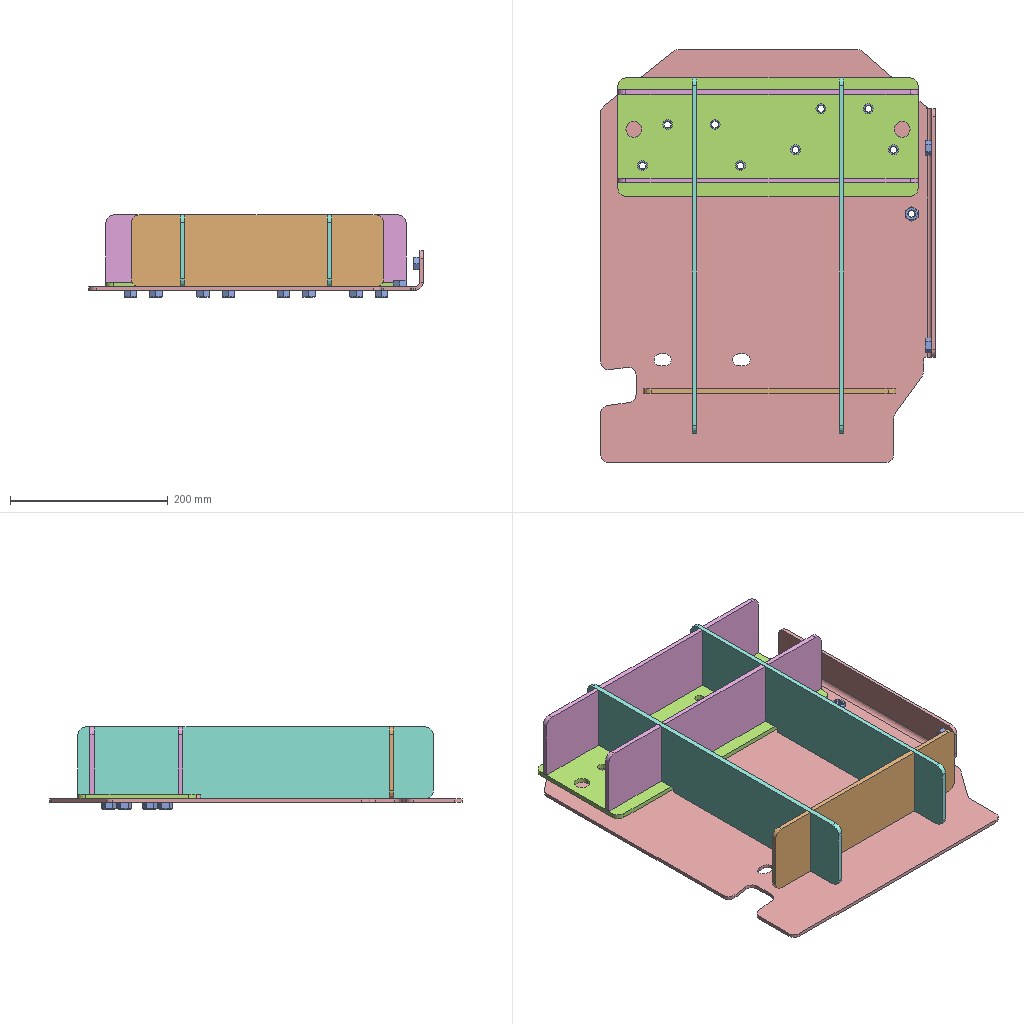Assembly | SolidWorks | 6 different items | 18 placed | box 424 x 523 x 104 mm
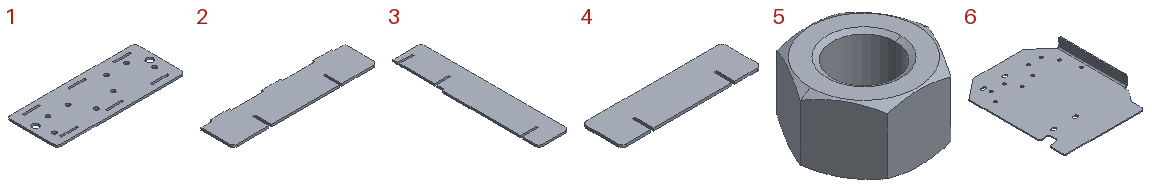Parts list (item | quantity | size | volume | features):
1 | x1 | 380 x 150 x 6 mm | 321025 mm3 | features FlatPattern 1, SMBaseFlange 1, SheetMetal 1
2 | x2 | 380 x 90.5 x 6 mm | 195432 mm3 | features FlatPattern 1, SMBaseFlange 1, SheetMetal 1
3 | x2 | 91 x 450 x 6 mm | 234874 mm3 | features FlatPattern 1, SMBaseFlange 1, SheetMetal 1
4 | x1 | 320 x 91 x 6 mm | 171145 mm3 | features Fillet 1, FlatPattern 1, SMBaseFlange 1, SheetMetal 1
5 | x11 | 27.713 x 24 x 14.8 mm | 5071 mm3 | features RevCut 2, Chamfer 1, Extrusion 1, LPattern 1
6 | x1 | 424 x 523 x 50 mm | 979518 mm3 | features EdgeFlange 1, Fillet 1, FlatPattern 1, ICE 1, SMBaseFlange 1, SheetMetal 1
Mates (type | each side: item.copy, entity, surface, feature):
Concentric | 6.1 face cylinder Base-Flange1 | 5.1 face cone EndChamfer
Coincident | 6.1 face plane Base-Flange1 | 5.1 face plane BaseNut
Parallel | 6.1 face plane Edge-Flange1 | 5.1 face plane BaseNut
Concentric | 6.1 face cylinder Cut-Extrude1 | 5.2 face cone EndChamfer
Coincident | 6.1 face plane Edge-Flange1 | 5.2 face plane BaseNut
Parallel | 6.1 face plane Edge-Flange1 | 5.2 face plane BaseNut
Concentric | 6.1 face cylinder Cut-Extrude1 | 5.3 face cone EndChamfer
Coincident | 6.1 face plane Edge-Flange1 | 5.3 face plane BaseNut
Parallel | 6.1 face plane Edge-Flange1 | 5.3 face plane BaseNut
Concentric | 6.1 face cylinder Base-Flange1 | 5.4 face cone EndChamfer
Coincident | 6.1 face plane Base-Flange1 | 5.4 face plane BaseNut
Parallel | 6.1 face plane Edge-Flange1 | 5.4 face plane BaseNut
Concentric | 6.1 face cylinder Base-Flange1 | 5.5 face cone EndChamfer
Coincident | 6.1 face plane Base-Flange1 | 5.5 face plane BaseNut
Concentric | 6.1 face cylinder Base-Flange1 | 5.6 face cone EndChamfer
Coincident | 6.1 face plane Base-Flange1 | 5.6 face plane BaseNut
Concentric | 6.1 face cylinder Base-Flange1 | 5.7 face cone EndChamfer
Coincident | 6.1 face plane Base-Flange1 | 5.7 face plane BaseNut
Concentric | 6.1 face cylinder Base-Flange1 | 5.8 face cone EndChamfer
Coincident | 6.1 face plane Base-Flange1 | 5.8 face plane BaseNut
Concentric | 6.1 face cylinder Base-Flange1 | 5.9 face cone EndChamfer
Coincident | 6.1 face plane Base-Flange1 | 5.9 face plane BaseNut
Concentric | 6.1 face cylinder Base-Flange1 | 5.10 face cone EndChamfer
Coincident | 6.1 face plane Base-Flange1 | 5.10 face plane BaseNut
Concentric | 6.1 face cylinder Base-Flange1 | 5.11 face cone EndChamfer
Coincident | 6.1 face plane Base-Flange1 | 5.11 face plane BaseNut
Parallel | 6.1 face plane Edge-Flange1 | 5.6 face plane BaseNut
Parallel | 6.1 face plane Edge-Flange1 | 5.5 face plane BaseNut
Parallel | 6.1 face plane Edge-Flange1 | 5.7 face plane BaseNut
Parallel | 6.1 face plane Edge-Flange1 | 5.8 face plane BaseNut
Parallel | 6.1 face plane Edge-Flange1 | 5.10 face plane BaseNut
Parallel | 6.1 face plane Edge-Flange1 | 5.9 face plane BaseNut
Parallel | 6.1 face plane Edge-Flange1 | 5.11 face plane BaseNut
InPlace | 6.1 face plane Base-Flange1 | 1.1 plane
InPlace | 2.1 plane | assembly plane
InPlace | 3.1 plane | assembly plane
InPlace | 4.1 plane | assembly plane